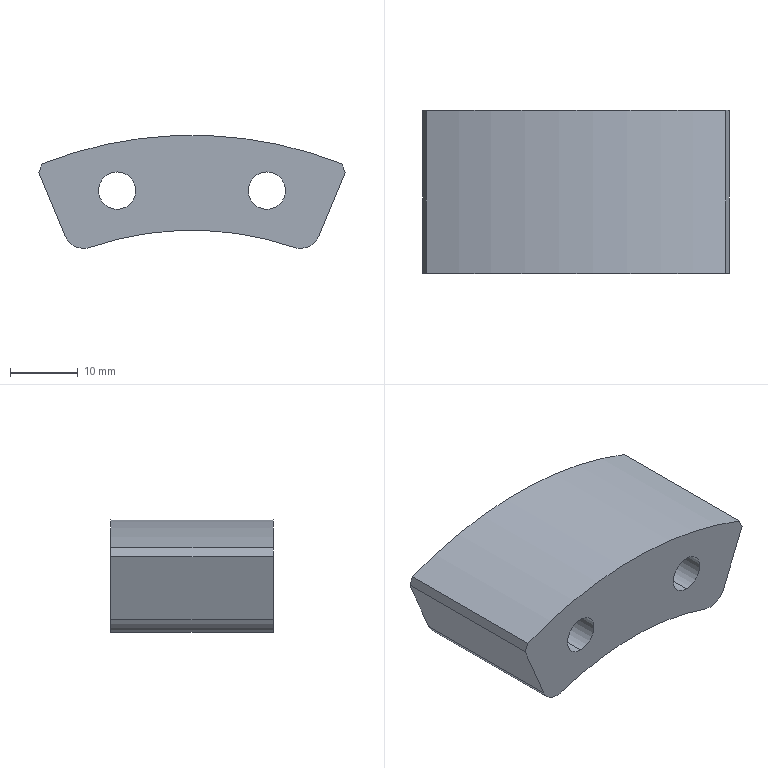Part | SolidWorks | features Chamfer 1, Extrusion 1, Fillet 1, HoleWzd 1, ICE 1 | 1 solid | 22 faces | box 45.157 x 24 x 16.667 mm | volume 11971 mm3 | cylinder 14 | plane 8 | commonest cylinder face diameters 5.5 x4 6 x4 10 x4 92 x1 120 x1
STEP:
#1=CARTESIAN_POINT('',(-11.019,17.,46.842));
#2=VERTEX_POINT('',#1);
#3=CARTESIAN_POINT('',(-11.019,17.,56.842));
#4=VERTEX_POINT('',#3);
#5=CARTESIAN_POINT('',(-11.019,17.,51.842));
#6=DIRECTION('',(0.,1.,0.));
#7=DIRECTION('',(0.,0.,1.));
#8=AXIS2_PLACEMENT_3D('',#5,#6,#7);
#9=CIRCLE('',#8,5.);
#10=EDGE_CURVE('',#2,#4,#9,.T.);
#11=ORIENTED_EDGE('',*,*,#10,.F.);
#12=CARTESIAN_POINT('',(-11.019,24.,46.842));
#13=VERTEX_POINT('',#12);
#14=CARTESIAN_POINT('',(-11.019,24.,46.842));
#15=DIRECTION('',(0.,1.,0.));
#16=VECTOR('',#15,1000.);
#17=LINE('',#14,#16);
#18=EDGE_CURVE('',#2,#13,#17,.T.);
#19=ORIENTED_EDGE('',*,*,#18,.T.);
#20=CARTESIAN_POINT('',(-11.019,24.,56.842));
#21=VERTEX_POINT('',#20);
#22=CARTESIAN_POINT('',(-11.019,24.,51.842));
#23=DIRECTION('',(0.,1.,0.));
#24=DIRECTION('',(0.,0.,1.));
#25=AXIS2_PLACEMENT_3D('',#22,#23,#24);
#26=CIRCLE('',#25,5.);
#27=EDGE_CURVE('',#13,#21,#26,.T.);
#28=ORIENTED_EDGE('',*,*,#27,.T.);
#29=CARTESIAN_POINT('',(-11.019,24.,56.842));
#30=DIRECTION('',(0.,1.,0.));
#31=VECTOR('',#30,1000.);
#32=LINE('',#29,#31);
#33=EDGE_CURVE('',#4,#21,#32,.T.);
#34=ORIENTED_EDGE('',*,*,#33,.F.);
#35=EDGE_LOOP('',(#11,#19,#28,#34));
#36=FACE_OUTER_BOUND('',#35,.T.);
#37=CARTESIAN_POINT('',(-11.019,24.,51.842));
#38=DIRECTION('',(0.,1.,0.));
#39=DIRECTION('',(0.,0.,1.));
#40=AXIS2_PLACEMENT_3D('',#37,#38,#39);
#41=CYLINDRICAL_SURFACE('',#40,5.);
#42=ADVANCED_FACE('',(#36),#41,.F.);
#43=CARTESIAN_POINT('',(-11.019,0.,49.092));
#44=VERTEX_POINT('',#43);
#45=CARTESIAN_POINT('',(-11.019,0.,54.592));
#46=VERTEX_POINT('',#45);
#47=CARTESIAN_POINT('',(-11.019,0.,51.842));
#48=DIRECTION('',(0.,1.,0.));
#49=DIRECTION('',(0.,0.,1.));
#50=AXIS2_PLACEMENT_3D('',#47,#48,#49);
#51=CIRCLE('',#50,2.75);
#52=EDGE_CURVE('',#44,#46,#51,.T.);
#53=ORIENTED_EDGE('',*,*,#52,.F.);
#54=CARTESIAN_POINT('',(-11.019,17.,49.092));
#55=VERTEX_POINT('',#54);
#56=CARTESIAN_POINT('',(-11.019,24.,49.092));
#57=DIRECTION('',(0.,1.,0.));
#58=VECTOR('',#57,1000.);
#59=LINE('',#56,#58);
#60=EDGE_CURVE('',#44,#55,#59,.T.);
#61=ORIENTED_EDGE('',*,*,#60,.T.);
#62=CARTESIAN_POINT('',(-11.019,17.,54.592));
#63=VERTEX_POINT('',#62);
#64=CARTESIAN_POINT('',(-11.019,17.,51.842));
#65=DIRECTION('',(0.,1.,0.));
#66=DIRECTION('',(0.,0.,1.));
#67=AXIS2_PLACEMENT_3D('',#64,#65,#66);
#68=CIRCLE('',#67,2.75);
#69=EDGE_CURVE('',#55,#63,#68,.T.);
#70=ORIENTED_EDGE('',*,*,#69,.T.);
#71=CARTESIAN_POINT('',(-11.019,24.,54.592));
#72=DIRECTION('',(0.,1.,0.));
#73=VECTOR('',#72,1000.);
#74=LINE('',#71,#73);
#75=EDGE_CURVE('',#46,#63,#74,.T.);
#76=ORIENTED_EDGE('',*,*,#75,.F.);
#77=EDGE_LOOP('',(#53,#61,#70,#76));
#78=FACE_OUTER_BOUND('',#77,.T.);
#79=CARTESIAN_POINT('',(-11.019,24.,51.842));
#80=DIRECTION('',(0.,1.,0.));
#81=DIRECTION('',(0.,0.,1.));
#82=AXIS2_PLACEMENT_3D('',#79,#80,#81);
#83=CYLINDRICAL_SURFACE('',#82,2.75);
#84=ADVANCED_FACE('',(#78),#83,.F.);
#85=CARTESIAN_POINT('',(11.019,17.,46.842));
#86=VERTEX_POINT('',#85);
#87=CARTESIAN_POINT('',(11.019,17.,56.842));
#88=VERTEX_POINT('',#87);
#89=CARTESIAN_POINT('',(11.019,17.,51.842));
#90=DIRECTION('',(0.,1.,0.));
#91=DIRECTION('',(0.,0.,1.));
#92=AXIS2_PLACEMENT_3D('',#89,#90,#91);
#93=CIRCLE('',#92,5.);
#94=EDGE_CURVE('',#86,#88,#93,.T.);
#95=ORIENTED_EDGE('',*,*,#94,.F.);
#96=CARTESIAN_POINT('',(11.019,24.,46.842));
#97=VERTEX_POINT('',#96);
#98=CARTESIAN_POINT('',(11.019,24.,46.842));
#99=DIRECTION('',(0.,1.,0.));
#100=VECTOR('',#99,1000.);
#101=LINE('',#98,#100);
#102=EDGE_CURVE('',#86,#97,#101,.T.);
#103=ORIENTED_EDGE('',*,*,#102,.T.);
#104=CARTESIAN_POINT('',(11.019,24.,56.842));
#105=VERTEX_POINT('',#104);
#106=CARTESIAN_POINT('',(11.019,24.,51.842));
#107=DIRECTION('',(0.,1.,0.));
#108=DIRECTION('',(0.,0.,1.));
#109=AXIS2_PLACEMENT_3D('',#106,#107,#108);
#110=CIRCLE('',#109,5.);
#111=EDGE_CURVE('',#97,#105,#110,.T.);
#112=ORIENTED_EDGE('',*,*,#111,.T.);
#113=CARTESIAN_POINT('',(11.019,24.,56.842));
#114=DIRECTION('',(0.,1.,0.));
#115=VECTOR('',#114,1000.);
#116=LINE('',#113,#115);
#117=EDGE_CURVE('',#88,#105,#116,.T.);
#118=ORIENTED_EDGE('',*,*,#117,.F.);
#119=EDGE_LOOP('',(#95,#103,#112,#118));
#120=FACE_OUTER_BOUND('',#119,.T.);
#121=CARTESIAN_POINT('',(11.019,24.,51.842));
#122=DIRECTION('',(0.,1.,0.));
#123=DIRECTION('',(0.,0.,1.));
#124=AXIS2_PLACEMENT_3D('',#121,#122,#123);
#125=CYLINDRICAL_SURFACE('',#124,5.);
#126=ADVANCED_FACE('',(#120),#125,.F.);
#127=CARTESIAN_POINT('',(11.019,0.,49.092));
#128=VERTEX_POINT('',#127);
#129=CARTESIAN_POINT('',(11.019,0.,54.592));
#130=VERTEX_POINT('',#129);
#131=CARTESIAN_POINT('',(11.019,0.,51.842));
#132=DIRECTION('',(0.,1.,0.));
#133=DIRECTION('',(0.,0.,1.));
#134=AXIS2_PLACEMENT_3D('',#131,#132,#133);
#135=CIRCLE('',#134,2.75);
#136=EDGE_CURVE('',#128,#130,#135,.T.);
#137=ORIENTED_EDGE('',*,*,#136,.F.);
#138=CARTESIAN_POINT('',(11.019,17.,49.092));
#139=VERTEX_POINT('',#138);
#140=CARTESIAN_POINT('',(11.019,24.,49.092));
#141=DIRECTION('',(0.,1.,0.));
#142=VECTOR('',#141,1000.);
#143=LINE('',#140,#142);
#144=EDGE_CURVE('',#128,#139,#143,.T.);
#145=ORIENTED_EDGE('',*,*,#144,.T.);
#146=CARTESIAN_POINT('',(11.019,17.,54.592));
#147=VERTEX_POINT('',#146);
#148=CARTESIAN_POINT('',(11.019,17.,51.842));
#149=DIRECTION('',(0.,1.,0.));
#150=DIRECTION('',(0.,0.,1.));
#151=AXIS2_PLACEMENT_3D('',#148,#149,#150);
#152=CIRCLE('',#151,2.75);
#153=EDGE_CURVE('',#139,#147,#152,.T.);
#154=ORIENTED_EDGE('',*,*,#153,.T.);
#155=CARTESIAN_POINT('',(11.019,24.,54.592));
#156=DIRECTION('',(0.,1.,0.));
#157=VECTOR('',#156,1000.);
#158=LINE('',#155,#157);
#159=EDGE_CURVE('',#130,#147,#158,.T.);
#160=ORIENTED_EDGE('',*,*,#159,.F.);
#161=EDGE_LOOP('',(#137,#145,#154,#160));
#162=FACE_OUTER_BOUND('',#161,.T.);
#163=CARTESIAN_POINT('',(11.019,24.,51.842));
#164=DIRECTION('',(0.,1.,0.));
#165=DIRECTION('',(0.,0.,1.));
#166=AXIS2_PLACEMENT_3D('',#163,#164,#165);
#167=CYLINDRICAL_SURFACE('',#166,2.75);
#168=ADVANCED_FACE('',(#162),#167,.F.);
#169=CARTESIAN_POINT('',(15.945,24.,43.333));
#170=VERTEX_POINT('',#169);
#171=CARTESIAN_POINT('',(14.968,24.,43.496));
#172=VERTEX_POINT('',#171);
#173=CARTESIAN_POINT('',(15.945,24.,46.333));
#174=DIRECTION('',(0.,1.,0.));
#175=DIRECTION('',(0.,0.,1.));
#176=AXIS2_PLACEMENT_3D('',#173,#174,#175);
#177=CIRCLE('',#176,3.);
#178=EDGE_CURVE('',#170,#172,#177,.T.);
#179=ORIENTED_EDGE('',*,*,#178,.F.);
#180=CARTESIAN_POINT('',(15.945,0.,43.333));
#181=VERTEX_POINT('',#180);
#182=CARTESIAN_POINT('',(15.945,24.,43.333));
#183=DIRECTION('',(0.,-1.,0.));
#184=VECTOR('',#183,1000.);
#185=LINE('',#182,#184);
#186=EDGE_CURVE('',#170,#181,#185,.T.);
#187=ORIENTED_EDGE('',*,*,#186,.T.);
#188=CARTESIAN_POINT('',(14.968,0.,43.496));
#189=VERTEX_POINT('',#188);
#190=CARTESIAN_POINT('',(15.945,0.,46.333));
#191=DIRECTION('',(0.,-1.,0.));
#192=DIRECTION('',(0.,0.,1.));
#193=AXIS2_PLACEMENT_3D('',#190,#191,#192);
#194=CIRCLE('',#193,3.);
#195=EDGE_CURVE('',#189,#181,#194,.T.);
#196=ORIENTED_EDGE('',*,*,#195,.F.);
#197=CARTESIAN_POINT('',(14.968,24.,43.496));
#198=DIRECTION('',(0.,-1.,0.));
#199=VECTOR('',#198,1000.);
#200=LINE('',#197,#199);
#201=EDGE_CURVE('',#172,#189,#200,.T.);
#202=ORIENTED_EDGE('',*,*,#201,.F.);
#203=EDGE_LOOP('',(#179,#187,#196,#202));
#204=FACE_OUTER_BOUND('',#203,.T.);
#205=CARTESIAN_POINT('',(15.945,24.,46.333));
#206=DIRECTION('',(0.,-1.,0.));
#207=DIRECTION('',(0.,0.,-1.));
#208=AXIS2_PLACEMENT_3D('',#205,#206,#207);
#209=CYLINDRICAL_SURFACE('',#208,3.);
#210=ADVANCED_FACE('',(#204),#209,.T.);
#211=CARTESIAN_POINT('',(-15.945,24.,43.333));
#212=VERTEX_POINT('',#211);
#213=CARTESIAN_POINT('',(-18.716,24.,45.185));
#214=VERTEX_POINT('',#213);
#215=CARTESIAN_POINT('',(-15.945,24.,46.333));
#216=DIRECTION('',(0.,1.,0.));
#217=DIRECTION('',(0.,0.,1.));
#218=AXIS2_PLACEMENT_3D('',#215,#216,#217);
#219=CIRCLE('',#218,3.);
#220=EDGE_CURVE('',#212,#214,#219,.T.);
#221=ORIENTED_EDGE('',*,*,#220,.F.);
#222=CARTESIAN_POINT('',(-15.945,0.,43.333));
#223=VERTEX_POINT('',#222);
#224=CARTESIAN_POINT('',(-15.945,24.,43.333));
#225=DIRECTION('',(0.,-1.,0.));
#226=VECTOR('',#225,1000.);
#227=LINE('',#224,#226);
#228=EDGE_CURVE('',#212,#223,#227,.T.);
#229=ORIENTED_EDGE('',*,*,#228,.T.);
#230=CARTESIAN_POINT('',(-18.716,0.,45.185));
#231=VERTEX_POINT('',#230);
#232=CARTESIAN_POINT('',(-15.945,0.,46.333));
#233=DIRECTION('',(0.,-1.,0.));
#234=DIRECTION('',(0.,0.,1.));
#235=AXIS2_PLACEMENT_3D('',#232,#233,#234);
#236=CIRCLE('',#235,3.);
#237=EDGE_CURVE('',#231,#223,#236,.T.);
#238=ORIENTED_EDGE('',*,*,#237,.F.);
#239=CARTESIAN_POINT('',(-18.716,0.,45.185));
#240=DIRECTION('',(0.,-1.,0.));
#241=VECTOR('',#240,1000.);
#242=LINE('',#239,#241);
#243=EDGE_CURVE('',#214,#231,#242,.T.);
#244=ORIENTED_EDGE('',*,*,#243,.F.);
#245=EDGE_LOOP('',(#221,#229,#238,#244));
#246=FACE_OUTER_BOUND('',#245,.T.);
#247=CARTESIAN_POINT('',(-15.945,24.,46.333));
#248=DIRECTION('',(0.,-1.,0.));
#249=DIRECTION('',(0.,0.,-1.));
#250=AXIS2_PLACEMENT_3D('',#247,#248,#249);
#251=CYLINDRICAL_SURFACE('',#250,3.);
#252=ADVANCED_FACE('',(#246),#251,.T.);
#253=CARTESIAN_POINT('',(-11.019,24.,51.842));
#254=DIRECTION('',(0.,1.,0.));
#255=DIRECTION('',(0.,0.,1.));
#256=AXIS2_PLACEMENT_3D('',#253,#254,#255);
#257=CIRCLE('',#256,5.);
#258=EDGE_CURVE('',#21,#13,#257,.T.);
#259=ORIENTED_EDGE('',*,*,#258,.F.);
#260=ORIENTED_EDGE('',*,*,#27,.F.);
#261=EDGE_LOOP('',(#259,#260));
#262=FACE_BOUND('',#261,.T.);
#263=CARTESIAN_POINT('',(11.019,24.,51.842));
#264=DIRECTION('',(0.,1.,0.));
#265=DIRECTION('',(0.,0.,1.));
#266=AXIS2_PLACEMENT_3D('',#263,#264,#265);
#267=CIRCLE('',#266,5.);
#268=EDGE_CURVE('',#105,#97,#267,.T.);
#269=ORIENTED_EDGE('',*,*,#268,.F.);
#270=ORIENTED_EDGE('',*,*,#111,.F.);
#271=EDGE_LOOP('',(#269,#270));
#272=FACE_BOUND('',#271,.T.);
#273=CARTESIAN_POINT('',(-22.578,24.,54.509));
#274=VERTEX_POINT('',#273);
#275=CARTESIAN_POINT('',(-17.603,24.,42.498));
#276=DIRECTION('',(-0.3827,0.,0.9239));
#277=VECTOR('',#276,1000.);
#278=LINE('',#275,#277);
#279=EDGE_CURVE('',#214,#274,#278,.T.);
#280=ORIENTED_EDGE('',*,*,#279,.T.);
#281=CARTESIAN_POINT('',(-22.042,24.,55.805));
#282=VERTEX_POINT('',#281);
#283=CARTESIAN_POINT('',(-38.544,24.,15.965));
#284=DIRECTION('',(0.3827,0.,0.9239));
#285=VECTOR('',#284,1000.);
#286=LINE('',#283,#285);
#287=EDGE_CURVE('',#274,#282,#286,.T.);
#288=ORIENTED_EDGE('',*,*,#287,.T.);
#289=CARTESIAN_POINT('',(22.042,24.,55.805));
#290=VERTEX_POINT('',#289);
#291=CARTESIAN_POINT('',(0.,24.,0.));
#292=DIRECTION('',(0.,1.,0.));
#293=DIRECTION('',(0.,0.,1.));
#294=AXIS2_PLACEMENT_3D('',#291,#292,#293);
#295=CIRCLE('',#294,60.);
#296=EDGE_CURVE('',#282,#290,#295,.T.);
#297=ORIENTED_EDGE('',*,*,#296,.T.);
#298=CARTESIAN_POINT('',(22.578,24.,54.509));
#299=VERTEX_POINT('',#298);
#300=CARTESIAN_POINT('',(38.544,24.,15.965));
#301=DIRECTION('',(0.3827,0.,-0.9239));
#302=VECTOR('',#301,1000.);
#303=LINE('',#300,#302);
#304=EDGE_CURVE('',#290,#299,#303,.T.);
#305=ORIENTED_EDGE('',*,*,#304,.T.);
#306=CARTESIAN_POINT('',(18.716,24.,45.185));
#307=VERTEX_POINT('',#306);
#308=CARTESIAN_POINT('',(17.603,24.,42.498));
#309=DIRECTION('',(-0.3827,0.,-0.9239));
#310=VECTOR('',#309,1000.);
#311=LINE('',#308,#310);
#312=EDGE_CURVE('',#299,#307,#311,.T.);
#313=ORIENTED_EDGE('',*,*,#312,.T.);
#314=CARTESIAN_POINT('',(15.945,24.,46.333));
#315=DIRECTION('',(0.,1.,0.));
#316=DIRECTION('',(0.,0.,1.));
#317=AXIS2_PLACEMENT_3D('',#314,#315,#316);
#318=CIRCLE('',#317,3.);
#319=EDGE_CURVE('',#307,#170,#318,.T.);
#320=ORIENTED_EDGE('',*,*,#319,.T.);
#321=ORIENTED_EDGE('',*,*,#178,.T.);
#322=CARTESIAN_POINT('',(-14.968,24.,43.496));
#323=VERTEX_POINT('',#322);
#324=CARTESIAN_POINT('',(0.,24.,0.));
#325=DIRECTION('',(0.,1.,0.));
#326=DIRECTION('',(0.,0.,1.));
#327=AXIS2_PLACEMENT_3D('',#324,#325,#326);
#328=CIRCLE('',#327,46.);
#329=EDGE_CURVE('',#323,#172,#328,.T.);
#330=ORIENTED_EDGE('',*,*,#329,.F.);
#331=CARTESIAN_POINT('',(-15.945,24.,46.333));
#332=DIRECTION('',(0.,1.,0.));
#333=DIRECTION('',(0.,0.,1.));
#334=AXIS2_PLACEMENT_3D('',#331,#332,#333);
#335=CIRCLE('',#334,3.);
#336=EDGE_CURVE('',#323,#212,#335,.T.);
#337=ORIENTED_EDGE('',*,*,#336,.T.);
#338=ORIENTED_EDGE('',*,*,#220,.T.);
#339=EDGE_LOOP('',(#280,#288,#297,#305,#313,#320,#321,#330,#337,#338));
#340=FACE_OUTER_BOUND('',#339,.T.);
#341=CARTESIAN_POINT('',(0.,24.,0.));
#342=DIRECTION('',(0.,1.,0.));
#343=DIRECTION('',(0.,0.,1.));
#344=AXIS2_PLACEMENT_3D('',#341,#342,#343);
#345=PLANE('',#344);
#346=ADVANCED_FACE('',(#262,#272,#340),#345,.T.);
#347=CARTESIAN_POINT('',(-11.019,0.,51.842));
#348=DIRECTION('',(0.,1.,0.));
#349=DIRECTION('',(0.,0.,1.));
#350=AXIS2_PLACEMENT_3D('',#347,#348,#349);
#351=CIRCLE('',#350,2.75);
#352=EDGE_CURVE('',#46,#44,#351,.T.);
#353=ORIENTED_EDGE('',*,*,#352,.T.);
#354=ORIENTED_EDGE('',*,*,#52,.T.);
#355=EDGE_LOOP('',(#353,#354));
#356=FACE_BOUND('',#355,.T.);
#357=CARTESIAN_POINT('',(11.019,0.,51.842));
#358=DIRECTION('',(0.,1.,0.));
#359=DIRECTION('',(0.,0.,1.));
#360=AXIS2_PLACEMENT_3D('',#357,#358,#359);
#361=CIRCLE('',#360,2.75);
#362=EDGE_CURVE('',#130,#128,#361,.T.);
#363=ORIENTED_EDGE('',*,*,#362,.T.);
#364=ORIENTED_EDGE('',*,*,#136,.T.);
#365=EDGE_LOOP('',(#363,#364));
#366=FACE_BOUND('',#365,.T.);
#367=CARTESIAN_POINT('',(-22.042,0.,55.805));
#368=VERTEX_POINT('',#367);
#369=CARTESIAN_POINT('',(22.042,0.,55.805));
#370=VERTEX_POINT('',#369);
#371=CARTESIAN_POINT('',(0.,0.,0.));
#372=DIRECTION('',(0.,1.,0.));
#373=DIRECTION('',(0.,0.,1.));
#374=AXIS2_PLACEMENT_3D('',#371,#372,#373);
#375=CIRCLE('',#374,60.);
#376=EDGE_CURVE('',#368,#370,#375,.T.);
#377=ORIENTED_EDGE('',*,*,#376,.F.);
#378=CARTESIAN_POINT('',(-22.578,0.,54.509));
#379=VERTEX_POINT('',#378);
#380=CARTESIAN_POINT('',(-22.578,0.,54.509));
#381=DIRECTION('',(-0.3827,0.,-0.9239));
#382=VECTOR('',#381,1000.);
#383=LINE('',#380,#382);
#384=EDGE_CURVE('',#368,#379,#383,.T.);
#385=ORIENTED_EDGE('',*,*,#384,.T.);
#386=CARTESIAN_POINT('',(-17.603,0.,42.498));
#387=DIRECTION('',(-0.3827,0.,0.9239));
#388=VECTOR('',#387,1000.);
#389=LINE('',#386,#388);
#390=EDGE_CURVE('',#231,#379,#389,.T.);
#391=ORIENTED_EDGE('',*,*,#390,.F.);
#392=ORIENTED_EDGE('',*,*,#237,.T.);
#393=CARTESIAN_POINT('',(-14.968,0.,43.496));
#394=VERTEX_POINT('',#393);
#395=CARTESIAN_POINT('',(-15.945,0.,46.333));
#396=DIRECTION('',(0.,-1.,0.));
#397=DIRECTION('',(0.,0.,1.));
#398=AXIS2_PLACEMENT_3D('',#395,#396,#397);
#399=CIRCLE('',#398,3.);
#400=EDGE_CURVE('',#223,#394,#399,.T.);
#401=ORIENTED_EDGE('',*,*,#400,.T.);
#402=CARTESIAN_POINT('',(0.,0.,0.));
#403=DIRECTION('',(0.,1.,0.));
#404=DIRECTION('',(0.,0.,1.));
#405=AXIS2_PLACEMENT_3D('',#402,#403,#404);
#406=CIRCLE('',#405,46.);
#407=EDGE_CURVE('',#394,#189,#406,.T.);
#408=ORIENTED_EDGE('',*,*,#407,.T.);
#409=ORIENTED_EDGE('',*,*,#195,.T.);
#410=CARTESIAN_POINT('',(18.716,0.,45.185));
#411=VERTEX_POINT('',#410);
#412=CARTESIAN_POINT('',(15.945,0.,46.333));
#413=DIRECTION('',(0.,-1.,0.));
#414=DIRECTION('',(0.,0.,1.));
#415=AXIS2_PLACEMENT_3D('',#412,#413,#414);
#416=CIRCLE('',#415,3.);
#417=EDGE_CURVE('',#181,#411,#416,.T.);
#418=ORIENTED_EDGE('',*,*,#417,.T.);
#419=CARTESIAN_POINT('',(22.578,0.,54.509));
#420=VERTEX_POINT('',#419);
#421=CARTESIAN_POINT('',(17.603,0.,42.498));
#422=DIRECTION('',(-0.3827,0.,-0.9239));
#423=VECTOR('',#422,1000.);
#424=LINE('',#421,#423);
#425=EDGE_CURVE('',#420,#411,#424,.T.);
#426=ORIENTED_EDGE('',*,*,#425,.F.);
#427=CARTESIAN_POINT('',(22.042,0.,55.805));
#428=DIRECTION('',(-0.3827,0.,0.9239));
#429=VECTOR('',#428,1000.);
#430=LINE('',#427,#429);
#431=EDGE_CURVE('',#420,#370,#430,.T.);
#432=ORIENTED_EDGE('',*,*,#431,.T.);
#433=EDGE_LOOP('',(#377,#385,#391,#392,#401,#408,#409,#418,#426,#432));
#434=FACE_OUTER_BOUND('',#433,.T.);
#435=CARTESIAN_POINT('',(0.,0.,0.));
#436=DIRECTION('',(0.,1.,0.));
#437=DIRECTION('',(0.,0.,1.));
#438=AXIS2_PLACEMENT_3D('',#435,#436,#437);
#439=PLANE('',#438);
#440=ADVANCED_FACE('',(#356,#366,#434),#439,.F.);
#441=ORIENTED_EDGE('',*,*,#296,.F.);
#442=CARTESIAN_POINT('',(-22.042,24.,55.805));
#443=DIRECTION('',(0.,-1.,0.));
#444=VECTOR('',#443,1000.);
#445=LINE('',#442,#444);
#446=EDGE_CURVE('',#282,#368,#445,.T.);
#447=ORIENTED_EDGE('',*,*,#446,.T.);
#448=ORIENTED_EDGE('',*,*,#376,.T.);
#449=CARTESIAN_POINT('',(22.042,24.,55.805));
#450=DIRECTION('',(0.,1.,0.));
#451=VECTOR('',#450,1000.);
#452=LINE('',#449,#451);
#453=EDGE_CURVE('',#370,#290,#452,.T.);
#454=ORIENTED_EDGE('',*,*,#453,.T.);
#455=EDGE_LOOP('',(#441,#447,#448,#454));
#456=FACE_OUTER_BOUND('',#455,.T.);
#457=CARTESIAN_POINT('',(0.,24.,0.));
#458=DIRECTION('',(0.,-1.,0.));
#459=DIRECTION('',(0.,0.,-1.));
#460=AXIS2_PLACEMENT_3D('',#457,#458,#459);
#461=CYLINDRICAL_SURFACE('',#460,60.);
#462=ADVANCED_FACE('',(#456),#461,.T.);
#463=ORIENTED_EDGE('',*,*,#407,.F.);
#464=CARTESIAN_POINT('',(-14.968,24.,43.496));
#465=DIRECTION('',(0.,1.,0.));
#466=VECTOR('',#465,1000.);
#467=LINE('',#464,#466);
#468=EDGE_CURVE('',#394,#323,#467,.T.);
#469=ORIENTED_EDGE('',*,*,#468,.T.);
#470=ORIENTED_EDGE('',*,*,#329,.T.);
#471=ORIENTED_EDGE('',*,*,#201,.T.);
#472=EDGE_LOOP('',(#463,#469,#470,#471));
#473=FACE_OUTER_BOUND('',#472,.T.);
#474=CARTESIAN_POINT('',(0.,24.,0.));
#475=DIRECTION('',(0.,-1.,0.));
#476=DIRECTION('',(0.,0.,-1.));
#477=AXIS2_PLACEMENT_3D('',#474,#475,#476);
#478=CYLINDRICAL_SURFACE('',#477,46.);
#479=ADVANCED_FACE('',(#473),#478,.F.);
#480=ORIENTED_EDGE('',*,*,#312,.F.);
#481=CARTESIAN_POINT('',(22.578,0.,54.509));
#482=DIRECTION('',(0.,-1.,0.));
#483=VECTOR('',#482,1000.);
#484=LINE('',#481,#483);
#485=EDGE_CURVE('',#299,#420,#484,.T.);
#486=ORIENTED_EDGE('',*,*,#485,.T.);
#487=ORIENTED_EDGE('',*,*,#425,.T.);
#488=CARTESIAN_POINT('',(18.716,0.,45.185));
#489=DIRECTION('',(0.,1.,0.));
#490=VECTOR('',#489,1000.);
#491=LINE('',#488,#490);
#492=EDGE_CURVE('',#411,#307,#491,.T.);
#493=ORIENTED_EDGE('',*,*,#492,.T.);
#494=EDGE_LOOP('',(#480,#486,#487,#493));
#495=FACE_OUTER_BOUND('',#494,.T.);
#496=CARTESIAN_POINT('',(17.603,0.,42.498));
#497=DIRECTION('',(0.9239,0.,-0.3827));
#498=DIRECTION('',(-0.3827,0.,-0.9239));
#499=AXIS2_PLACEMENT_3D('',#496,#497,#498);
#500=PLANE('',#499);
#501=ADVANCED_FACE('',(#495),#500,.T.);
#502=ORIENTED_EDGE('',*,*,#390,.T.);
#503=CARTESIAN_POINT('',(-22.578,24.,54.509));
#504=DIRECTION('',(0.,1.,0.));
#505=VECTOR('',#504,1000.);
#506=LINE('',#503,#505);
#507=EDGE_CURVE('',#379,#274,#506,.T.);
#508=ORIENTED_EDGE('',*,*,#507,.T.);
#509=ORIENTED_EDGE('',*,*,#279,.F.);
#510=ORIENTED_EDGE('',*,*,#243,.T.);
#511=EDGE_LOOP('',(#502,#508,#509,#510));
#512=FACE_OUTER_BOUND('',#511,.T.);
#513=CARTESIAN_POINT('',(-17.603,0.,42.498));
#514=DIRECTION('',(-0.9239,0.,-0.3827));
#515=DIRECTION('',(-0.3827,0.,0.9239));
#516=AXIS2_PLACEMENT_3D('',#513,#514,#515);
#517=PLANE('',#516);
#518=ADVANCED_FACE('',(#512),#517,.T.);
#519=ORIENTED_EDGE('',*,*,#228,.F.);
#520=ORIENTED_EDGE('',*,*,#336,.F.);
#521=ORIENTED_EDGE('',*,*,#468,.F.);
#522=ORIENTED_EDGE('',*,*,#400,.F.);
#523=EDGE_LOOP('',(#519,#520,#521,#522));
#524=FACE_OUTER_BOUND('',#523,.T.);
#525=CARTESIAN_POINT('',(-15.945,24.,46.333));
#526=DIRECTION('',(0.,-1.,0.));
#527=DIRECTION('',(0.,0.,-1.));
#528=AXIS2_PLACEMENT_3D('',#525,#526,#527);
#529=CYLINDRICAL_SURFACE('',#528,3.);
#530=ADVANCED_FACE('',(#524),#529,.T.);
#531=ORIENTED_EDGE('',*,*,#186,.F.);
#532=ORIENTED_EDGE('',*,*,#319,.F.);
#533=ORIENTED_EDGE('',*,*,#492,.F.);
#534=ORIENTED_EDGE('',*,*,#417,.F.);
#535=EDGE_LOOP('',(#531,#532,#533,#534));
#536=FACE_OUTER_BOUND('',#535,.T.);
#537=CARTESIAN_POINT('',(15.945,24.,46.333));
#538=DIRECTION('',(0.,-1.,0.));
#539=DIRECTION('',(0.,0.,-1.));
#540=AXIS2_PLACEMENT_3D('',#537,#538,#539);
#541=CYLINDRICAL_SURFACE('',#540,3.);
#542=ADVANCED_FACE('',(#536),#541,.T.);
#543=ORIENTED_EDGE('',*,*,#384,.F.);
#544=ORIENTED_EDGE('',*,*,#446,.F.);
#545=ORIENTED_EDGE('',*,*,#287,.F.);
#546=ORIENTED_EDGE('',*,*,#507,.F.);
#547=EDGE_LOOP('',(#543,#544,#545,#546));
#548=FACE_OUTER_BOUND('',#547,.T.);
#549=CARTESIAN_POINT('',(-22.578,24.,54.509));
#550=DIRECTION('',(-0.9239,0.,0.3827));
#551=DIRECTION('',(0.,-1.,0.));
#552=AXIS2_PLACEMENT_3D('',#549,#550,#551);
#553=PLANE('',#552);
#554=ADVANCED_FACE('',(#548),#553,.T.);
#555=ORIENTED_EDGE('',*,*,#431,.F.);
#556=ORIENTED_EDGE('',*,*,#485,.F.);
#557=ORIENTED_EDGE('',*,*,#304,.F.);
#558=ORIENTED_EDGE('',*,*,#453,.F.);
#559=EDGE_LOOP('',(#555,#556,#557,#558));
#560=FACE_OUTER_BOUND('',#559,.T.);
#561=CARTESIAN_POINT('',(22.042,24.,55.805));
#562=DIRECTION('',(0.9239,0.,0.3827));
#563=DIRECTION('',(0.,-1.,0.));
#564=AXIS2_PLACEMENT_3D('',#561,#562,#563);
#565=PLANE('',#564);
#566=ADVANCED_FACE('',(#560),#565,.T.);
#567=ORIENTED_EDGE('',*,*,#144,.F.);
#568=ORIENTED_EDGE('',*,*,#362,.F.);
#569=ORIENTED_EDGE('',*,*,#159,.T.);
#570=CARTESIAN_POINT('',(11.019,17.,51.842));
#571=DIRECTION('',(0.,1.,0.));
#572=DIRECTION('',(0.,0.,1.));
#573=AXIS2_PLACEMENT_3D('',#570,#571,#572);
#574=CIRCLE('',#573,2.75);
#575=EDGE_CURVE('',#147,#139,#574,.T.);
#576=ORIENTED_EDGE('',*,*,#575,.T.);
#577=EDGE_LOOP('',(#567,#568,#569,#576));
#578=FACE_OUTER_BOUND('',#577,.T.);
#579=CARTESIAN_POINT('',(11.019,24.,51.842));
#580=DIRECTION('',(0.,1.,0.));
#581=DIRECTION('',(0.,0.,1.));
#582=AXIS2_PLACEMENT_3D('',#579,#580,#581);
#583=CYLINDRICAL_SURFACE('',#582,2.75);
#584=ADVANCED_FACE('',(#578),#583,.F.);
#585=ORIENTED_EDGE('',*,*,#575,.F.);
#586=ORIENTED_EDGE('',*,*,#153,.F.);
#587=EDGE_LOOP('',(#585,#586));
#588=FACE_BOUND('',#587,.T.);
#589=CARTESIAN_POINT('',(11.019,17.,51.842));
#590=DIRECTION('',(0.,1.,0.));
#591=DIRECTION('',(0.,0.,1.));
#592=AXIS2_PLACEMENT_3D('',#589,#590,#591);
#593=CIRCLE('',#592,5.);
#594=EDGE_CURVE('',#88,#86,#593,.T.);
#595=ORIENTED_EDGE('',*,*,#594,.T.);
#596=ORIENTED_EDGE('',*,*,#94,.T.);
#597=EDGE_LOOP('',(#595,#596));
#598=FACE_OUTER_BOUND('',#597,.T.);
#599=CARTESIAN_POINT('',(13.769,17.,51.842));
#600=DIRECTION('',(0.,-1.,0.));
#601=DIRECTION('',(0.,0.,-1.));
#602=AXIS2_PLACEMENT_3D('',#599,#600,#601);
#603=PLANE('',#602);
#604=ADVANCED_FACE('',(#588,#598),#603,.F.);
#605=ORIENTED_EDGE('',*,*,#102,.F.);
#606=ORIENTED_EDGE('',*,*,#594,.F.);
#607=ORIENTED_EDGE('',*,*,#117,.T.);
#608=ORIENTED_EDGE('',*,*,#268,.T.);
#609=EDGE_LOOP('',(#605,#606,#607,#608));
#610=FACE_OUTER_BOUND('',#609,.T.);
#611=CARTESIAN_POINT('',(11.019,24.,51.842));
#612=DIRECTION('',(0.,1.,0.));
#613=DIRECTION('',(0.,0.,1.));
#614=AXIS2_PLACEMENT_3D('',#611,#612,#613);
#615=CYLINDRICAL_SURFACE('',#614,5.);
#616=ADVANCED_FACE('',(#610),#615,.F.);
#617=ORIENTED_EDGE('',*,*,#60,.F.);
#618=ORIENTED_EDGE('',*,*,#352,.F.);
#619=ORIENTED_EDGE('',*,*,#75,.T.);
#620=CARTESIAN_POINT('',(-11.019,17.,51.842));
#621=DIRECTION('',(0.,1.,0.));
#622=DIRECTION('',(0.,0.,1.));
#623=AXIS2_PLACEMENT_3D('',#620,#621,#622);
#624=CIRCLE('',#623,2.75);
#625=EDGE_CURVE('',#63,#55,#624,.T.);
#626=ORIENTED_EDGE('',*,*,#625,.T.);
#627=EDGE_LOOP('',(#617,#618,#619,#626));
#628=FACE_OUTER_BOUND('',#627,.T.);
#629=CARTESIAN_POINT('',(-11.019,24.,51.842));
#630=DIRECTION('',(0.,1.,0.));
#631=DIRECTION('',(0.,0.,1.));
#632=AXIS2_PLACEMENT_3D('',#629,#630,#631);
#633=CYLINDRICAL_SURFACE('',#632,2.75);
#634=ADVANCED_FACE('',(#628),#633,.F.);
#635=ORIENTED_EDGE('',*,*,#625,.F.);
#636=ORIENTED_EDGE('',*,*,#69,.F.);
#637=EDGE_LOOP('',(#635,#636));
#638=FACE_BOUND('',#637,.T.);
#639=CARTESIAN_POINT('',(-11.019,17.,51.842));
#640=DIRECTION('',(0.,1.,0.));
#641=DIRECTION('',(0.,0.,1.));
#642=AXIS2_PLACEMENT_3D('',#639,#640,#641);
#643=CIRCLE('',#642,5.);
#644=EDGE_CURVE('',#4,#2,#643,.T.);
#645=ORIENTED_EDGE('',*,*,#644,.T.);
#646=ORIENTED_EDGE('',*,*,#10,.T.);
#647=EDGE_LOOP('',(#645,#646));
#648=FACE_OUTER_BOUND('',#647,.T.);
#649=CARTESIAN_POINT('',(-8.269,17.,51.842));
#650=DIRECTION('',(0.,-1.,0.));
#651=DIRECTION('',(0.,0.,-1.));
#652=AXIS2_PLACEMENT_3D('',#649,#650,#651);
#653=PLANE('',#652);
#654=ADVANCED_FACE('',(#638,#648),#653,.F.);
#655=ORIENTED_EDGE('',*,*,#18,.F.);
#656=ORIENTED_EDGE('',*,*,#644,.F.);
#657=ORIENTED_EDGE('',*,*,#33,.T.);
#658=ORIENTED_EDGE('',*,*,#258,.T.);
#659=EDGE_LOOP('',(#655,#656,#657,#658));
#660=FACE_OUTER_BOUND('',#659,.T.);
#661=CARTESIAN_POINT('',(-11.019,24.,51.842));
#662=DIRECTION('',(0.,1.,0.));
#663=DIRECTION('',(0.,0.,1.));
#664=AXIS2_PLACEMENT_3D('',#661,#662,#663);
#665=CYLINDRICAL_SURFACE('',#664,5.);
#666=ADVANCED_FACE('',(#660),#665,.F.);
#667=CLOSED_SHELL('',(#42,#84,#126,#168,#210,#252,#346,#440,#462,#479,#501,#518,#530,#542,#554,#566,#584,#604,#616,#634,#654,#666));
#668=MANIFOLD_SOLID_BREP('',#667);
#669=CARTESIAN_POINT('',(0.,0.,0.));
#670=DIRECTION('',(0.,0.,1.));
#671=DIRECTION('',(1.,0.,0.));
#672=AXIS2_PLACEMENT_3D('',#669,#670,#671);
#673=(LENGTH_UNIT()NAMED_UNIT(*)SI_UNIT(.MILLI.,.METRE.));
#674=UNCERTAINTY_MEASURE_WITH_UNIT(LENGTH_MEASURE(0.00001),#673,'','');
#675=(NAMED_UNIT(*)PLANE_ANGLE_UNIT()SI_UNIT($,.RADIAN.));
#676=(NAMED_UNIT(*)SI_UNIT($,.STERADIAN.)SOLID_ANGLE_UNIT());
#677=(GEOMETRIC_REPRESENTATION_CONTEXT(3)GLOBAL_UNCERTAINTY_ASSIGNED_CONTEXT((#674))GLOBAL_UNIT_ASSIGNED_CONTEXT((#673,#675,#676))REPRESENTATION_CONTEXT('',''));
#678=ADVANCED_BREP_SHAPE_REPRESENTATION('',(#668,#672),#677);